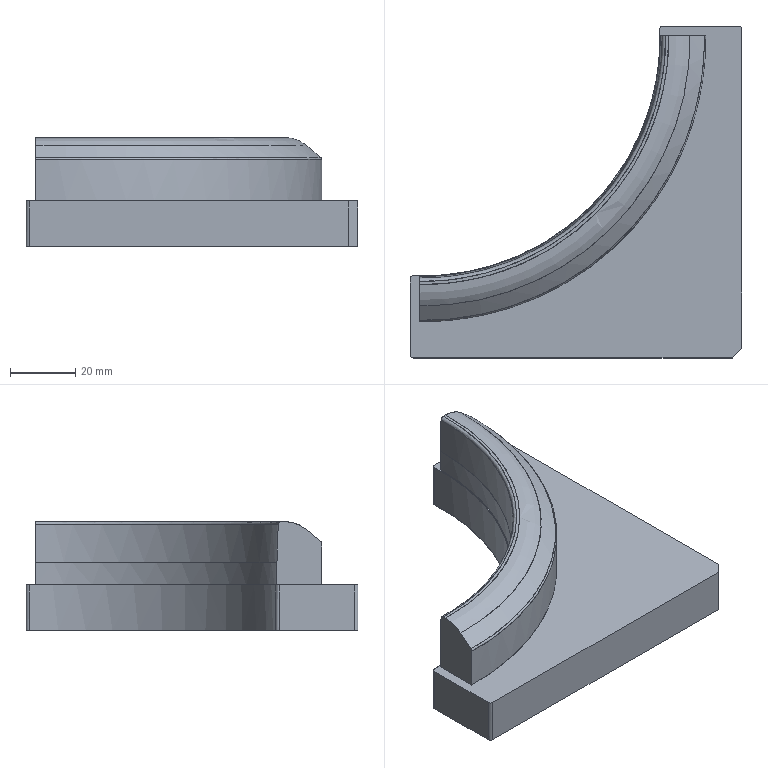NC program | PowerMill | posted with a generic post | part box 102 x 102 x 33.478 mm
Lines 1 to 929 of 205885:
%
O0001
N104 ( POWERMILL CB  : 2026004.0)
N105 ( POST VER      : 2026.0.0.5161)
N106 ( OPTION FILE   : FANUC)
N107 ( OUTPUT WORKPLANE : WORLD)
N108 (  )
N109 ( TOOL LIST )
N110 (---------------------------------------)
N111 ( NO. | ID        | DIA.| TIP RAD|LENGTH)
N112 (---------------------------------------)
N113 (    1|D10C_1_1_1 |10.0 |  0.0   |88.92 )
N114 (    3|D10_1_1_1  |10.0 |  0.0   |88.64 )
N115 (    7|R2_2_1_1   | 4.0 |  2.0   |69.64 )
N116 (   13|TEXT_D4_1_1| 4.0 |  0.3   |74.72 )
N117 (---------------------------------------)
N118 (  )
N119 ( NUMBER OF TOOLPATHS: 11.0 )
N120 ( ESTIMATED PROGRAM DURATION: 0 HOURS 57 MIN 41 SEC)
N121 (  )
N122 G00 G21 G80 G40 G17
N123 G90
N124 G54
N125 G53 Z0.0
N126 (---------------)
N127 ( START TOOLPATH : 粗公开粗01-扫面平行-D10C )
N128 (---------------)
N129 ( TOOL NO.    :1 )
N130 ( TOOL TYPE   : ENDMILL)
N131 ( TOOL ID     : D10C_1_1_1)
N132 ( TOOL DIA    : 10.0 LENGTH 88.92)
N133 T1
N134 M6
N135 S8000 M03
N136 G00 G90 X0.0 Y0.0
N137 G43 Z10.2 H1
N138
N139 G05 P10000 R4
N140 X63.7 Y58.7
N141 Z1.199
N142 G01 Z-0.001 F6000.0
N143 X58.7 F10000.0
N144 X-58.7
N145 Y52.83
N146 X58.7
N147 Y46.96
N148 X-58.7
N149 Y41.09
N150 X58.7
N151 Y35.22
N152 X-58.7
N153 Y29.35
N154 X58.7
N155 Y23.48
N156 X-58.7
N157 Y17.61
N158 X58.7
N159 Y11.74
N160 X-58.7
N161 Y5.87
N162 X58.7
N163 Y0.0
N164 X-58.7
N165 Y-5.87
N166 X58.7
N167 Y-11.74
N168 X-58.7
N169 Y-17.61
N170 X58.7
N171 Y-23.48
N172 X-58.7
N173 Y-29.35
N174 X58.7
N175 Y-35.22
N176 X-58.7
N177 Y-41.09
N178 X58.7
N179 Y-46.96
N180 X-58.7
N181 Y-52.83
N182 X58.7
N183 Y-58.7
N184 X-58.7
N185 X-63.7
N186 Z-0.202
N187 X-58.7
N188 X58.7
N189 Y-52.83
N190 X-58.7
N191 Y-46.96
N192 X58.7
N193 Y-41.09
N194 X-58.7
N195 Y-35.22
N196 X58.7
N197 Y-29.35
N198 X-58.7
N199 Y-23.48
N200 X58.7
N201 Y-17.61
N202 X-58.7
N203 Y-11.74
N204 X58.7
N205 Y-5.87
N206 X-58.7
N207 Y0.0
N208 X58.7
N209 Y5.87
N210 X-58.7
N211 Y11.74
N212 X58.7
N213 Y17.61
N214 X-58.7
N215 Y23.48
N216 X58.7
N217 Y29.35
N218 X-58.7
N219 Y35.22
N220 X58.7
N221 Y41.09
N222 X-58.7
N223 Y46.96
N224 X58.7
N225 Y52.83
N226 X-58.7
N227 Y58.7
N228 X58.7
N229 X63.7
N230 G00 Z10.2
N231 G05 P0
N232 (---------------)
N233 ( END TOOLPATH : 粗公开粗01-扫面平行-D10C )
N234 (---------------)
N235 ( START TOOLPATH : 粗公开粗01-外形偏置-D10C )
N236 (---------------)
N237 G00 X0.0 Y0.0 Z9.7984
N238 G05 P10000 R4
N239 X-63.975 Y-33.7508
N240 Z0.5546
N241 G01 Z-0.6454 F6000.0
N242 X-63.4475 F10000.0
N243 G03 X-58.7 Y-29.0033 I0.0 J4.7475
N244 G01 Y58.7
N245 X58.7
N246 Y-58.7
N247 X-58.7
N248 Y-29.0033
N249 X-53.1498 Y-29.0035
N250 X-53.1497 Y-26.6832
N251 X-53.0849 Y-25.9098
N252 X-52.9797 Y-25.4077
N253 X-52.8987 Y-25.1364
N254 X-52.5774 Y-24.3629
N255 X-52.0889 Y-23.5895
N256 X-51.4329 Y-22.8817
N257 X-50.6594 Y-22.3105
N258 X-50.1536 Y-22.0427
N259 X-49.886 Y-21.9284
N260 X-49.1126 Y-21.6925
N261 X-48.3392 Y-21.5818
N262 X-45.2454 Y-21.5529
N263 X-42.9252 Y-21.4486
N264 X-39.8315 Y-21.1992
N265 X-36.7378 Y-20.7992
N266 X-34.4175 Y-20.41
N267 X-32.0972 Y-19.9294
N268 X-29.0035 Y-19.1725
N269 X-26.6832 Y-18.4912
N270 X-23.5895 Y-17.4552
N271 X-21.2692 Y-16.5643
N272 X-18.9489 Y-15.5709
N273 X-16.2797 Y-14.3084
N274 X-13.535 Y-12.8509
N275 X-11.2147 Y-11.4941
N276 X-8.8944 Y-10.0095
N277 X-6.5741 Y-8.3865
N278 X-5.0273 Y-7.2213
N279 X-2.707 Y-5.3478
N280 X-0.588 Y-3.4804
N281 X1.1601 Y-1.8086
N282 X3.2947 Y0.3867
N283 X5.0273 Y2.3321
N284 X6.6129 Y4.2538
N285 X8.3865 Y6.5741
N286 X10.0094 Y8.8944
N287 X11.4941 Y11.2147
N288 X11.5897 Y11.3783
N289 X6.0055 Y14.6704
N290 X0.4423 Y17.9501
N291 X-5.1295 Y21.2348
N292 X-10.7095 Y24.5244
N293 X-15.5015 Y27.3494
N294 G03 X-17.1054 Y29.9885 I-1.5092 J0.8897
N295 G01 X-27.5446 Y29.4236
N296 G03 X-29.4336 Y27.5359 I0.108 J-1.997
N297 G01 X-30.0063 Y17.0787
N298 G03 X-27.0213 Y15.7459 I1.7473 J-0.0957
N299 G01 X-15.7716 Y27.0005
N300 X-15.6255 Y27.1664
N301 X-15.5015 Y27.3494
N302 X-10.7095 Y24.5244
N303 X-10.4281 Y24.9783
N304 X-10.1522 Y25.4355
N305 X-5.8027 Y32.7447
N306 G03 X-7.5635 Y35.767 I-1.7187 J1.0228
N307 G01 X-33.2745 Y35.2262
N308 G03 X-35.232 Y33.2701 I0.042 J-1.9996
N309 G01 X-35.7919 Y7.5289
N310 G03 X-32.7684 Y5.7674 I1.9996 J-0.0435
N311 G01 X-25.4451 Y10.1321
N312 G03 X-10.7095 Y24.5244 I-22.5386 J37.8161
N313 G01 X-5.1295 Y21.2348
N314 G03 X-0.3815 Y31.0923 I-42.8543 J26.7134
N315 G01 X2.3491 Y38.8039
N316 G03 X0.4437 Y41.4713 I-1.8853 J0.6676
N317 G01 X-39.096 Y41.0734
N318 G03 X-41.0757 Y39.0948 I0.0202 J-1.9999
N319 G01 X-41.498 Y-0.5049
N320 G03 X-38.8241 Y-2.4092 I1.9999 J-0.0213
N321 G01 X-30.965 Y0.404
N322 G03 X-5.1295 Y21.2348 I-17.0187 J47.5442
N323 G01 X0.4423 Y17.9501
N324 G03 X7.8155 Y36.7357 I-48.1713 J29.7466
N325 G01 X9.4205 Y44.8691
N326 G03 X7.4462 Y47.2563 I-1.9621 J0.3872
N327 G01 X-44.95 Y46.9375
N328 G03 X-46.9378 Y44.9504 I0.0121 J-2.0
N329 G01 X-47.2756 Y-7.5891
N330 G03 X-44.8632 Y-9.559 I1.9999 J-0.0129
N331 G01 X-36.0513 Y-7.7015
N332 G03 X0.4423 Y17.9501 I-11.6777 J55.3982
N333 G01 X6.0055 Y14.6704
N334 G02 X-38.7348 Y-14.572 I-53.144 J32.4623
N335 G01 X-50.8237 Y-16.2184
N336 G02 X-53.0936 Y-14.2279 I-0.2699 J1.9817
N337 G01 X-52.8092 Y50.8179
N338 G02 X-50.8178 Y52.8092 I2.0 J-0.0087
N339 G01 X14.2352 Y53.0899
N340 G02 X16.2139 Y50.7453 I0.0086 J-2.0
N341 G01 X15.5005 Y46.6672
N342 G03 X15.0141 Y42.9866 I43.7629 J-7.6556
N343 G01 X14.886 Y41.561
N344 G02 X6.0055 Y14.6704 I-62.0245 J5.5717
N345 G01 X11.5897 Y11.3783
N346 X12.8508 Y13.535
N347 X14.3084 Y16.2792
N348 X15.571 Y18.9489
N349 X16.5643 Y21.2692
N350 X17.4543 Y23.5895
N351 X18.4926 Y26.6832
N352 X19.1721 Y29.0035
N353 X19.7549 Y31.3238
N354 X20.41 Y34.4175
N355 X20.7992 Y36.7378
N356 X21.1987 Y39.8315
N357 X21.4007 Y42.1517
N358 X21.4011 Y42.1612
N359 X21.5529 Y45.2454
N360 X21.5817 Y48.3392
N361 X21.6923 Y49.1126
N362 X21.9293 Y49.886
N363 X22.0427 Y50.1535
N364 X22.3104 Y50.6594
N365 X22.8161 Y51.358
N366 X23.5895 Y52.0887
N367 X24.3629 Y52.5785
N368 X25.1364 Y52.8986
N369 X25.4077 Y52.9797
N370 X25.9098 Y53.0845
N371 X26.6832 Y53.1497
N372 X31.3238 Y53.1498
N373 X32.0972 Y53.0827
N374 X32.5942 Y52.9797
N375 X32.8706 Y52.8956
N376 X33.6441 Y52.5715
N377 X34.2531 Y52.2063
N378 X35.12 Y51.4329
N379 X35.686 Y50.6594
N380 X36.0731 Y49.886
N381 X36.3093 Y49.1126
N382 X36.4157 Y48.3392
N383 X36.4096 Y46.0189
N384 X36.3438 Y43.6986
N385 X36.2195 Y41.3783
N386 X35.9643 Y38.3257
N387 X35.6817 Y35.9643
N388 X35.3362 Y33.6441
N389 X34.9221 Y31.3238
N390 X34.4175 Y28.8669
N391 X33.7046 Y25.9098
N392 X33.0632 Y23.5895
N393 X32.5892 Y22.0427
N394 X31.8215 Y19.7224
N395 X30.6899 Y16.6287
N396 X29.7769 Y14.3872
N397 X29.0588 Y12.7615
N398 X27.9731 Y10.4413
N399 X26.6832 Y7.8993
N400 X25.5293 Y5.8007
N401 X24.3629 Y3.8135
N402 X22.8161 Y1.3495
N403 X21.6465 Y-0.3867
N404 X19.9862 Y-2.707
N405 X18.8078 Y-4.2538
N406 X17.5692 Y-5.8007
N407 X15.6051 Y-8.121
N408 X13.4839 Y-10.4413
N409 X11.9881 Y-11.9741
N410 X11.9704 Y-11.9914
N411 X15.876 Y-15.8923
N412 X19.3672 Y-19.3794
N413 X22.9505 Y-22.9583
N414 X26.8594 Y-26.8626
N415 X30.0433 Y-30.0426
N416 X26.8594 Y-26.8626
N417 G02 X19.637 Y-33.4429 I-73.4321 J73.3439
N418 G01 X18.1502 Y-34.6746
N419 G03 X19.0834 Y-37.1455 I0.8907 J-1.0753
N420 G01 X34.7312 Y-36.6699
N421 G03 X36.6695 Y-34.7314 I-0.0608 J1.9991
N422 G01 X37.1449 Y-19.0569
N423 G03 X34.675 Y-18.1262 I-1.3944 J0.0423
N424 G01 X33.446 Y-19.6141
N425 G02 X26.8594 Y-26.8626 I-80.0197 J66.0962
N426 G01 X22.9505 Y-22.9583
N427 G02 X0.1995 Y-39.9582 I-69.8778 J69.7936
N428 G01 X-1.1305 Y-40.6804
N429 G03 X-0.5818 Y-42.8107 I0.541 J-0.9964
N430 G01 X40.5449 Y-42.5314
N431 G03 X42.5313 Y-40.545 I-0.0136 J1.9999
N432 G01 X42.8096 Y0.6258
N433 G03 X40.6799 Y1.1748 I-1.1337 J0.0077
N434 G01 X39.8955 Y-0.2683
N435 G02 X33.3408 Y-10.707 I-86.1713 J46.8327
N436 G01 X33.247 Y-10.8372
N437 G02 X22.9505 Y-22.9583 I-80.1743 J57.6726
N438 G01 X19.3672 Y-19.3794
N439 G02 X-25.597 Y-44.4026 I-66.2945 J66.2148
N440 G01 X-34.9541 Y-46.5902
N441 G02 X-47.3071 Y-47.3212 I-8.2986 J35.4964
N442 G01 X-47.6385 Y-47.2841
N443 G03 X-47.9693 Y-47.5637 I-0.0332 J-0.2962
N444 G03 X-47.6717 Y-47.8784 I0.2976 J-0.0166
N445 G01 X47.3749 Y-47.8828
N446 G03 X47.8828 Y-47.3749 I0.0 J0.5079
N447 G01 X47.8761 Y47.5041
N448 G03 X47.5297 Y47.987 I-0.5098 J0.0
N449 G01 X47.5032 Y47.996
N450 G03 X46.8687 Y47.5415 I-0.1541 J-0.4551
N451 G01 X46.8679 Y46.9182
N452 G02 X27.7547 Y-9.7505 I-93.9086 J0.1159
N453 G01 X27.7005 Y-9.8219
N454 G02 X19.3672 Y-19.3794 I-74.6278 J56.6573
N455 G01 X15.876 Y-15.8923
N456 X15.8874 Y-15.8808
N457 X15.8989 Y-15.8693
N458 X15.9859 Y-15.7821
N459 G03 X41.942 Y47.5765 I-63.0357 J62.8199
N460 G01 X41.9363 Y48.5244
N461 X41.7595 Y50.9481
N462 G02 X43.8356 Y53.0958 I1.9944 J0.1493
N463 G01 X50.8908 Y52.8075
N464 G02 X52.8092 Y50.8092 I-0.0816 J-1.9983
N465 G01 Y-50.8092
N466 G02 X50.8092 Y-52.8092 I-2.0 J0.0
N467 G01 X-50.8092
N468 G02 X-52.8075 Y-50.8903 I0.0 J2.0
N469 G01 X-53.094 Y-43.8335
N470 G02 X-50.7907 Y-41.7758 I1.9983 J0.0811
N471 G01 X-47.485 Y-42.2859
N472 G03 X-36.7548 Y-41.8984 I4.3534 J28.2109
N473 G01 X-27.0332 Y-39.6703
N474 G03 X15.876 Y-15.8923 I-19.7783 J86.2968
N475 G01 X11.9704 Y-11.9914
N476 X10.389 Y-13.535
N477 X8.7084 Y-15.0818
N478 X6.5741 Y-16.9339
N479 X5.0273 Y-18.1963
N480 X3.0559 Y-19.7224
N481 X0.9273 Y-21.2692
N482 X-1.3485 Y-22.8161
N483 X-3.4804 Y-24.1611
N484 X-5.0273 Y-25.0797
N485 X-7.3476 Y-26.3843
N486 X-9.6678 Y-27.5903
N487 X-11.9881 Y-28.7102
N488 X-14.3894 Y-29.7769
N489 X-16.6287 Y-30.6882
N490 X-18.9489 Y-31.5554
N491 X-21.2692 Y-32.3482
N492 X-23.5895 Y-33.0618
N493 X-25.6889 Y-33.6441
N494 X-28.2301 Y-34.2731
N495 X-30.5503 Y-34.7748
N496 X-32.8706 Y-35.2061
N497 X-35.9643 Y-35.6823
N498 X-38.3458 Y-35.9643
N499 X-40.6049 Y-36.168
N500 X-42.9252 Y-36.3149
N501 X-45.2454 Y-36.3927
N502 X-48.3392 Y-36.4194
N503 X-49.1126 Y-36.3055
N504 X-49.886 Y-36.0738
N505 X-50.6594 Y-35.6916
N506 X-51.4329 Y-35.1164
N507 X-52.2063 Y-34.2529
N508 X-52.5734 Y-33.6441
N509 X-52.8966 Y-32.8706
N510 X-52.9797 Y-32.5942
N511 X-53.0828 Y-32.0972
N512 X-53.1499 Y-31.3238
N513 X-53.1498 Y-29.0035
N514 X-58.7 Y-29.0033
N515 G00 Z3.2112
N516 G01 X-63.975 Y-33.7508
N517 G00 Z0.1612
N518 G01 Z-1.0388 F6000.0
N519 X-63.4475 F10000.0
N520 G03 X-58.7 Y-29.0033 I0.0 J4.7475
N521 G01 Y58.7
N522 X29.39
N523 X29.3902 Y53.15
N524 X32.0972 Y53.1501
N525 X32.8706 Y53.1289
N526 X33.6441 Y52.9996
N527 X34.4175 Y52.7422
N528 X35.1909 Y52.333
N529 X35.3804 Y52.2063
N530 X35.9643 Y51.725
N531 X36.2459 Y51.4329
N532 X36.8189 Y50.6594
N533 X37.2004 Y49.886
N534 X37.4372 Y49.1126
N535 X37.5476 Y48.3392
N536 X37.5517 Y46.0189
N537 X37.4604 Y42.9252
N538 X37.3184 Y40.6049
N539 X37.1089 Y38.2846
N540 X36.834 Y35.9643
N541 X36.4942 Y33.6441
N542 X35.9643 Y30.6509
N543 X35.4508 Y28.2301
N544 X34.8878 Y25.9098
N545 X34.2538 Y23.5895
N546 X33.5455 Y21.2692
N547 X32.7689 Y18.9489
N548 X31.9145 Y16.6287
N549 X30.9817 Y14.3084
N550 X29.9684 Y11.9881
N551 X29.0035 Y9.9455
N552 X27.686 Y7.3476
N553 X26.4071 Y5.0273
N554 X25.1364 Y2.88
N555 X24.0521 Y1.1601
N556 X22.5042 Y-1.1601
N557 X20.8365 Y-3.4804
N558 X19.7224 Y-4.9401
N559 X18.1755 Y-6.868
N560 X16.4484 Y-8.8944
N561 X14.3084 Y-11.234
N562 X12.8243 Y-12.7615
N563 X12.7941 Y-12.7908
N564 X16.7044 Y-16.702
N565 X19.9595 Y-19.9578
N566 X23.5401 Y-23.5393
N567 X27.4463 Y-27.4464
N568 X30.6279 Y-30.6287
N569 X27.4463 Y-27.4464
N570 G02 X20.7147 Y-33.6128 I-73.9166 J73.9336
N571 G01 X19.234 Y-34.8548
N572 G03 X20.1826 Y-37.3257 I0.8994 J-1.0723
N573 G01 X34.8794 Y-36.8083
N574 G03 X36.8078 Y-34.8799 I-0.0703 J1.9987
N575 G01 X37.3246 Y-20.1889
N576 G03 X34.8533 Y-19.2398 I-1.399 J0.0492
N577 G01 X33.6108 Y-20.7203
N578 G02 X27.4463 Y-27.4464 I-80.0807 J67.2071
N579 G01 X23.5401 Y-23.5393
N580 G02 X1.6784 Y-40.0639 I-70.4055 J70.4217
N581 G01 X0.1549 Y-40.9145
N582 G03 X0.7213 Y-43.048 I0.5553 J-0.9945
N583 G01 X40.6765 Y-42.657
N584 G03 X42.6568 Y-40.6766 I-0.0196 J1.9999
N585 G01 X43.0459 Y-0.7412
N586 G03 X40.912 Y-0.1743 I-1.1393 J0.0111
N587 G01 X40.0606 Y-1.6976
N588 G02 X23.5401 Y-23.5393 I-86.9258 J48.5798
N589 G01 X19.9595 Y-19.9578
N590 G02 X-25.061 Y-45.0966 I-66.8851 J66.9004
N591 G01 X-30.699 Y-46.4359
N592 G03 X-30.4898 Y-48.2007 I0.2068 J-0.8703
N593 G01 X46.0031 Y-47.9978
N594 G03 X47.9978 Y-46.003 I-0.0053 J2.0
N595 G01 X48.2009 Y31.8764
N596 G03 X46.503 Y32.0265 I-0.8554 J0.0022
N597 G01 X46.2513 Y30.592
N598 G02 X19.9595 Y-19.9578 I-93.1769 J16.3506
N599 G01 X16.7044 Y-16.702
N600 G03 X43.0738 Y47.583 I-63.6457 J63.6581
N601 G01 X43.0671 Y48.5455
N602 X42.8871 Y50.9432
N603 G02 X44.9782 Y53.0947 I1.9941 J0.1538
N604 G01 X50.9062 Y52.8068
N605 G02 X52.8092 Y50.8092 I-0.097 J-1.9976
N606 G01 Y38.7779
N607 X48.3092
N608 X52.8092
N609 Y-50.8092
N610 G02 X50.8092 Y-52.8092 I-2.0 J0.0
N611 G01 X-50.8092
N612 G02 X-52.8068 Y-50.9059 I0.0 J2.0
N613 G01 X-53.0939 Y-44.9767
N614 G02 X-50.7982 Y-42.9023 I1.9977 J0.0967
N615 G01 X-47.3963 Y-43.415
N616 G03 X-35.9717 Y-42.9452 I4.4954 J29.8312
N617 G01 X-26.2655 Y-40.6546
N618 G03 X16.7044 Y-16.702 I-20.6758 J87.6106
N619 G01 X12.7941 Y-12.7908
N620 X11.2147 Y-14.3254
N621 X9.6678 Y-15.7545
N622 X7.3476 Y-17.7804
N623 X5.8007 Y-19.042
N624 X3.4804 Y-20.8365
N625 X1.8111 Y-22.0427
N626 X-0.3867 Y-23.547
N627 X-2.8798 Y-25.1364
N628 X-5.0273 Y-26.4076
N629 X-7.3476 Y-27.686
N630 X-9.6678 Y-28.8693
N631 X-11.5669 Y-29.7769
N632 X-13.3066 Y-30.5503
N633 X-15.8552 Y-31.6104
N634 X-18.1755 Y-32.4904
N635 X-20.4958 Y-33.2923
N636 X-22.8161 Y-34.0219
N637 X-25.1364 Y-34.6781
N638 X-28.2301 Y-35.45
N639 X-30.6509 Y-35.9643
N640 X-32.8706 Y-36.3681
N641 X-35.1909 Y-36.7258
N642 X-37.5112 Y-37.0202
N643 X-40.6049 Y-37.3169
N644 X-42.9252 Y-37.4582
N645 X-44.3695 Y-37.5112
N646 X-45.2454 Y-37.537
N647 X-48.3392 Y-37.5467
N648 X-49.1126 Y-37.4351
N649 X-49.886 Y-37.2009
N650 X-50.6594 Y-36.8182
N651 X-51.4329 Y-36.2462
N652 X-51.7252 Y-35.9643
N653 X-52.2063 Y-35.3804
N654 X-52.333 Y-35.1909
N655 X-52.7417 Y-34.4175
N656 X-52.9797 Y-33.7225
N657 X-53.1289 Y-32.8706
N658 X-53.1501 Y-32.0972
N659 X-53.1499 Y-26.6832
N660 X-53.1111 Y-25.9098
N661 X-52.9797 Y-25.2219
N662 X-52.6687 Y-24.3629
N663 X-52.2247 Y-23.5895
N664 X-51.5628 Y-22.8161
N665 X-51.4329 Y-22.6958
N666 X-50.6594 Y-22.1252
N667 X-49.886 Y-21.7428
N668 X-49.1126 Y-21.5064
N669 X-48.3392 Y-21.3965
N670 X-45.2454 Y-21.3738
N671 X-42.9494 Y-21.2692
N672 X-39.8315 Y-21.0189
N673 X-37.5112 Y-20.7278
N674 X-34.4175 Y-20.2284
N675 X-32.0972 Y-19.7464
N676 X-29.0035 Y-18.9869
N677 X-26.6832 Y-18.3045
N678 X-23.9763 Y-17.4021
N679 X-21.2692 Y-16.3724
N680 X-18.9489 Y-15.376
N681 X-16.6946 Y-14.3084
N682 X-13.738 Y-12.7615
N683 X-11.2147 Y-11.2819
N684 X-8.8944 Y-9.7915
N685 X-7.3476 Y-8.7205
N686 X-5.0273 Y-6.997
N687 X-2.707 Y-5.1163
N688 X-0.8578 Y-3.4804
N689 X1.1601 Y-1.5601
N690 X3.0464 Y0.3867
N691 X5.0273 Y2.6022
N692 X6.5741 Y4.4895
N693 X8.1622 Y6.5741
N694 X9.7915 Y8.8944
N695 X11.2819 Y11.2147
N696 X11.4704 Y11.5361
N697 X5.8397 Y14.8096
N698 X0.2535 Y18.0573
N699 X-5.3463 Y21.3128
N700 X-10.9466 Y24.5686
N701 X-15.7577 Y27.3656
N702 G03 X-17.3703 Y29.9963 I-1.5152 J0.8809
N703 G01 X-27.5411 Y29.4302
N704 G03 X-29.427 Y27.543 I0.1111 J-1.9969
N705 G01 X-29.9959 Y17.1844
N706 G03 X-27.0254 Y15.8691 I1.7343 J-0.0953
N707 G01 X-16.0254 Y27.0155
N708 X-15.8805 Y27.1821
N709 X-15.7577 Y27.3656
N710 X-10.9466 Y24.5686
N711 X-10.6902 Y24.9846
N712 X-10.4384 Y25.4035
N713 X-6.0708 Y32.7605
N714 G03 X-7.834 Y35.781 I-1.7198 J1.021
N715 G01 X-33.2708 Y35.2295
N716 G03 X-35.227 Y33.2731 I0.0434 J-1.9995
N717 G01 X-35.7811 Y7.5536
N718 G03 X-32.7417 Y5.8021 I1.9996 J-0.043
N719 G01 X-25.4141 Y10.2621
N720 G03 X-10.9466 Y24.5686 I-22.9022 J37.628
N721 G01 X-5.3463 Y21.3128
N722 G03 X-0.8146 Y30.675 I-42.97 J26.5773
N723 G01 X2.1302 Y38.8006
N724 G03 X0.2292 Y41.482 I-1.8803 J0.6815
N725 G01 X-39.0945 Y41.0748
N726 G03 X-41.0737 Y39.0952 I0.0207 J-1.9999
N727 G01 X-41.4747 Y-0.5652
N728 G03 X-38.7794 Y-2.4607 I1.9999 J-0.0203
N729 G01 X-30.7476 Y0.518
N730 G03 X-5.3463 Y21.3128 I-17.5687 J47.3722
N731 G01 X0.2535 Y18.0573
N732 G03 X7.5148 Y36.4051 I-48.5698 J29.8329
N733 G01 X9.2538 Y44.8588
N734 G03 X7.2825 Y47.2617 I-1.9589 J0.4029
N735 G01 X-44.9505 Y46.9381
N736 G03 X-46.9381 Y44.9501 I0.0124 J-2.0
N737 G01 X-47.2538 Y-7.614
N738 G03 X-44.8521 Y-9.5853 I2.0 J-0.012
N739 G01 X-36.8694 Y-7.9488
N740 G03 X0.2535 Y18.0573 I-11.4469 J55.839
N741 G01 X5.8397 Y14.8096
N742 G02 X-41.599 Y-15.1104 I-53.782 J32.705
N743 G01 X-50.8954 Y-16.052
N744 G02 X-53.0969 Y-14.0533 I-0.2016 J1.9898
N745 G01 X-52.8092 Y50.8181
N746 G02 X-50.8181 Y52.8092 I2.0 J-0.0089
N747 G01 X14.0523 Y53.0973
N748 G02 X16.0321 Y50.7573 I0.0089 J-2.0
N749 G01 X15.3786 Y46.969
N750 X15.1841 Y45.7196
N751 X15.0308 Y44.4646
N752 X14.6554 Y40.9076
N753 G02 X5.8397 Y14.8096 I-62.5977 J6.607
N754 G01 X11.4704 Y11.5361
N755 X12.7615 Y13.738
N756 X14.2769 Y16.6287
N757 X15.376 Y18.9489
N758 X16.3724 Y21.2692
N759 X17.2615 Y23.5895
N760 X18.1755 Y26.2643
N761 X18.9869 Y29.0035
N762 X19.5702 Y31.3238
N763 X20.2284 Y34.4175
N764 X20.6175 Y36.7378
N765 X21.0189 Y39.8315
N766 X21.0198 Y39.8421
N767 X21.2195 Y42.1517
N768 X21.3738 Y45.2454
N769 X21.396 Y48.3392
N770 X21.5064 Y49.1126
N771 X21.7429 Y49.886
N772 X22.1247 Y50.6594
N773 X22.6962 Y51.4329
N774 X22.8161 Y51.5628
N775 X23.5633 Y52.2063
N776 X24.3629 Y52.6689
N777 X25.1364 Y52.9547
N778 X25.9098 Y53.1119
N779 X26.6832 Y53.1499
N780 X29.3902 Y53.15
N781 X29.39 Y58.7
N782 X58.7
N783 Y-58.7
N784 X-58.7
N785 Y-29.0033
N786 G00 Z2.8177
N787 G01 X-63.975 Y-33.7508
N788 G00 Z-0.2323
N789 G01 Z-1.4323 F6000.0
N790 X-63.4475 F10000.0
N791 G03 X-58.7 Y-29.0033 I0.0 J4.7475
N792 G01 Y58.7
N793 X29.7768
N794 X29.7769 Y53.15
N795 X32.8706 Y53.1501
N796 X33.6441 Y53.1338
N797 X34.4175 Y53.0127
N798 X35.1909 Y52.7648
N799 X35.9643 Y52.3682
N800 X36.2117 Y52.2063
N801 X36.7378 Y51.7783
N802 X37.079 Y51.4329
N803 X37.5112 Y50.8755
N804 X37.6503 Y50.6594
N805 X38.0321 Y49.886
N806 X38.2685 Y49.1126
N807 X38.3789 Y48.3392
N808 X38.3816 Y46.0189
N809 X38.3191 Y43.6986
N810 X38.1492 Y40.6049
N811 X37.9403 Y38.2846
N812 X37.6684 Y35.9643
N813 X37.3318 Y33.6441
N814 X36.7895 Y30.5503
N815 X36.2992 Y28.2301
N816 X35.7401 Y25.9098
N817 X35.1126 Y23.5895
N818 X34.4145 Y21.2692
N819 X33.6437 Y18.9489
N820 X32.5045 Y15.8552
N821 X31.8759 Y14.3084
N822 X30.8739 Y11.9881
N823 X29.7769 Y9.6429
N824 X28.6172 Y7.3476
N825 X27.3554 Y5.0273
N826 X25.9098 Y2.5569
N827 X24.5401 Y0.3867
N828 X22.9735 Y-1.9336
N829 X21.8638 Y-3.4804
N830 X20.1067 Y-5.8007
N831 X18.9489 Y-7.2295
N832 X16.8752 Y-9.6678
N833 X15.4616 Y-11.2147
N834 X13.535 Y-13.2195
N835 X11.6264 Y-15.0818
N836 X9.6678 Y-16.8715
N837 X8.121 Y-18.2086
N838 X5.8007 Y-20.1046
N839 X4.2538 Y-21.2865
N840 X1.9336 Y-22.9733
N841 X0.3867 Y-24.0234
N842 X-1.9336 Y-25.5207
N843 X-4.2538 Y-26.9139
N844 X-6.6138 Y-28.2301
N845 X-8.8944 Y-29.4122
N846 X-11.2649 Y-30.5503
N847 X-13.535 Y-31.556
N848 X-15.8552 Y-32.5045
N849 X-18.1755 Y-33.3744
N850 X-20.4958 Y-34.1682
N851 X-22.8161 Y-34.8884
N852 X-25.1364 Y-35.5363
N853 X-28.2301 Y-36.2981
N854 X-30.5503 Y-36.7895
N855 X-32.8706 Y-37.2103
N856 X-35.1909 Y-37.5648
N857 X-37.5112 Y-37.8545
N858 X-40.6049 Y-38.1492
N859 X-42.8305 Y-38.2846
N860 X-46.0189 Y-38.3816
N861 X-48.3392 Y-38.3786
N862 X-49.0332 Y-38.2846
N863 X-49.886 Y-38.0323
N864 X-50.6594 Y-37.6488
N865 X-50.8765 Y-37.5112
N866 X-51.4329 Y-37.0786
N867 X-51.7782 Y-36.7378
N868 X-52.2063 Y-36.2102
N869 X-52.3687 Y-35.9643
N870 X-52.7651 Y-35.1909
N871 X-52.9797 Y-34.5526
N872 X-53.1338 Y-33.6441
N873 X-53.1501 Y-32.8706
N874 X-53.1499 Y-26.6832
N875 X-53.1164 Y-25.9098
N876 X-52.9797 Y-25.1836
N877 X-52.6847 Y-24.3629
N878 X-52.2502 Y-23.5895
N879 X-51.6016 Y-22.8161
N880 X-51.4329 Y-22.658
N881 X-50.6594 Y-22.0869
N882 X-49.886 Y-21.7054
N883 X-49.1126 Y-21.4695
N884 X-48.3392 Y-21.3585
N885 X-45.2454 Y-21.3298
N886 X-42.9252 Y-21.2237
N887 X-39.8315 Y-20.9743
N888 X-37.5112 Y-20.684
N889 X-34.4175 Y-20.1842
N890 X-31.3238 Y-19.5244
N891 X-29.0327 Y-18.9489
N892 X-26.4031 Y-18.1755
N893 X-24.1149 Y-17.4021
N894 X-21.2692 Y-16.3247
N895 X-18.9489 Y-15.3276
N896 X-16.6287 Y-14.2282
N897 X-13.8266 Y-12.7615
N898 X-11.9881 Y-11.6951
N899 X-9.6678 Y-10.2472
N900 X-7.3476 Y-8.6666
N901 X-5.0273 Y-6.9414
N902 X-2.707 Y-5.0589
N903 X-0.9248 Y-3.4804
N904 X1.1601 Y-1.4985
N905 X2.9847 Y0.3867
N906 X5.0273 Y2.669
N907 X6.5741 Y4.5597
N908 X8.1065 Y6.5741
N909 X9.7375 Y8.8944
N910 X11.2292 Y11.2147
N911 X11.2971 Y11.3304
N912 X5.683 Y14.6485
N913 X0.1167 Y17.9384
N914 X-5.4596 Y21.2342
N915 X-11.0364 Y24.5304
N916 X-15.8252 Y27.3607
N917 G03 X-17.4239 Y29.9898 I-1.5016 J0.8875
N918 G01 X-27.5524 Y29.4257
N919 G03 X-29.438 Y27.5419 I0.1112 J-1.9969
N920 G01 X-30.011 Y17.429
N921 G03 X-27.0367 Y16.0952 I1.7419 J-0.0987
N922 G01 X-16.0948 Y27.0135
N923 X-15.949 Y27.1786
N924 X-15.8252 Y27.3607
N925 X-11.0364 Y24.5304
N926 X-10.7525 Y24.9833
N927 X-10.4741 Y25.4397
N928 X-6.0802 Y32.7434
N929 G03 X-7.837 Y35.774 I-1.7138 J1.0311
N930 G01 X-33.2772 Y35.2265
N931 G03 X-35.2336 Y33.2718 I0.0431 J-1.9996
N932 G01 X-35.8038 Y7.8498
N933 G03 X-32.7753 Y6.09 I1.9995 J-0.0448
N934 G01 X-25.4419 Y10.4898
N935 G03 X-11.0364 Y24.5304 I-22.4897 J37.4844
N936 G01 X-5.4596 Y21.2342
N937 G03 X-0.7854 Y30.7655 I-42.4719 J26.7399
N938 G01 X2.1421 Y38.7859
N939 G03 X0.2431 Y41.4715 I-1.8788 J0.6857
N940 G01 X-39.0966 Y41.0736
N941 G03 X-41.0763 Y39.0955 I0.0202 J-1.9999
N942 G01 X-41.5047 Y-0.2547
N943 G03 X-38.8134 Y-2.1531 I1.9999 J-0.0218
N944 G01 X-30.58 Y0.8804
N945 G03 X-5.4596 Y21.2342 I-17.3516 J47.0938
N946 G01 X0.1167 Y17.9384
N947 G03 X7.6151 Y36.7777 I-48.0482 J30.0357
N948 G01 X9.2438 Y44.858
N949 G03 X7.2711 Y47.2531 I-1.9606 J0.3952
N950 G01 X-44.9502 Y46.938
N951 G03 X-46.9381 Y44.951 I0.0121 J-2.0
N952 G01 X-47.2773 Y-7.3853
N953 G03 X-44.8507 Y-9.3522 I1.9999 J-0.013
N954 G01 X-35.8423 Y-7.385
N955 G03 X0.1167 Y17.9384 I-12.0893 J55.3592
N956 G01 X5.683 Y14.6485
N957 G02 X-39.1763 Y-14.4359 I-53.2248 J32.9557
N958 G01 X-50.8294 Y-16.0073
N959 G02 X-53.0967 Y-14.0163 I-0.2673 J1.9821
N960 G01 X-52.8092 Y50.8181
N961 G02 X-50.818 Y52.8092 I2.0 J-0.0089
N962 G01 X14.0146 Y53.096
N963 G02 X15.9952 Y50.7611 I0.0089 J-1.9999
N964 G01 X15.3624 Y47.0362
N965 G03 X14.9631 Y43.8607 I36.5453 J-6.2086
N966 G01 X14.8499 Y42.482
N967 G02 X5.683 Y14.6485 I-62.3917 J5.1222
N968 G01 X11.2971 Y11.3304
N969 X12.7615 Y13.8266
N970 X13.8359 Y15.8552
N971 X15.0818 Y18.4161
N972 X16.3247 Y21.2692
N973 X17.2142 Y23.5895
N974 X18.1755 Y26.4032
N975 X18.9409 Y29.0035
N976 X19.5244 Y31.3238
N977 X20.1843 Y34.4175
N978 X20.5724 Y36.7378
N979 X20.9743 Y39.8315
N980 X21.1749 Y42.1517
N981 X21.3294 Y45.2454
N982 X21.3295 Y45.2556
N983 X21.3581 Y48.3392
N984 X21.4695 Y49.1126
N985 X21.7047 Y49.886
N986 X22.0427 Y50.5848
N987 X22.658 Y51.4329
N988 X22.8161 Y51.6011
N989 X23.5263 Y52.2063
N990 X24.3629 Y52.6848
N991 X25.1364 Y52.9659
N992 X25.9098 Y53.1164
N993 X26.6832 Y53.1499
N994 X29.7769 Y53.15
N995 X29.7768 Y58.7
N996 X58.7
N997 Y-58.7
N998 X32.1902
N999 X31.9649 Y-52.8092
N1000 X31.7824 Y-48.0378
N1001 X31.5802 Y-42.7511
N1002 X31.3581 Y-36.9459
N1003 X31.1861 Y-32.4492
N1004 X31.3581 Y-36.9459
N1005 X34.8884 Y-36.8108
N1006 G03 X36.8105 Y-34.8887 I-0.0765 J1.9985
N1007 G01 X37.3218 Y-21.5106
N1008 G03 X34.8436 Y-20.541 I-1.4077 J0.0538
N1009 G01 X33.5851 Y-22.0122
N1010 G02 X22.0107 Y-33.5861 I-80.0365 J68.4656
N1011 G01 X20.5395 Y-34.8445
N1012 G03 X21.509 Y-37.3226 I0.9156 J-1.0705
N1013 G01 X31.3581 Y-36.9459
N1014 X31.5802 Y-42.7511
N1015 X40.6781 Y-42.6576
N1016 G03 X42.6575 Y-40.6782 I-0.0205 J1.9999
N1017 G01 X43.0487 Y-2.4819
N1018 G03 X40.9029 Y-1.8938 I-1.1503 J0.0118
N1019 G01 X40.0232 Y-3.4134
N1020 G02 X3.409 Y-40.0249 I-86.9381 J50.3303
N1021 G01 X1.8894 Y-40.9045
N1022 G03 X2.4774 Y-43.0502 I0.5762 J-0.9955
N1023 G01 X31.5802 Y-42.7511
N1024 X31.7824 Y-48.0378
N1025 X46.0034 Y-47.9978
N1026 G03 X47.9978 Y-46.0033 I-0.0056 J2.0